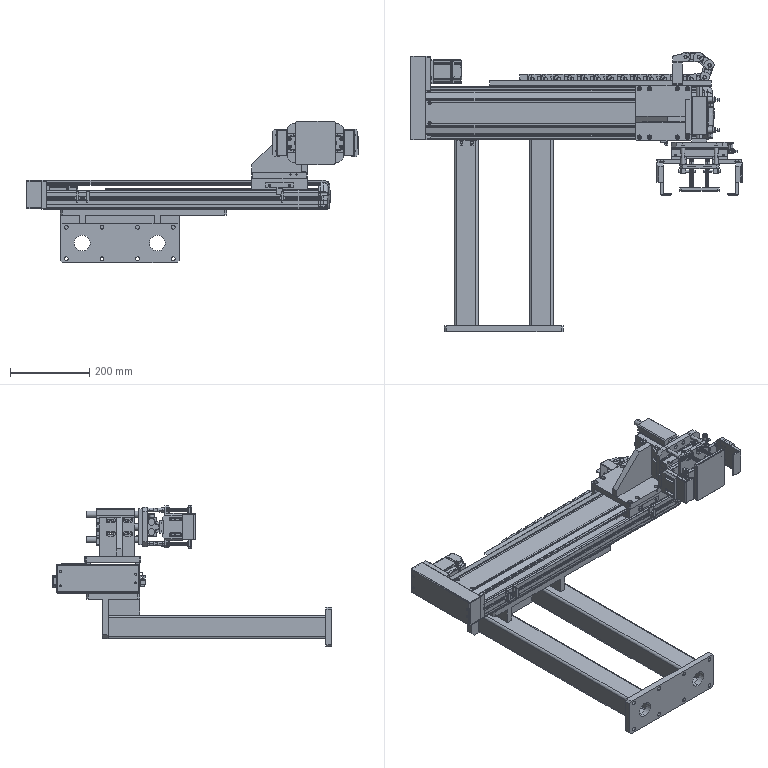Part | SolidWorks | 92 solids | 6352 faces | volume 8279258 mm3 | plane 3215 | cylinder 2463 | spline 353 | cone 283 | torus 26 | sphere 12 | commonest cylinder face diameters 2 x251 1 x193 0.6 x142 8 x122 4 x103 11.94 x96